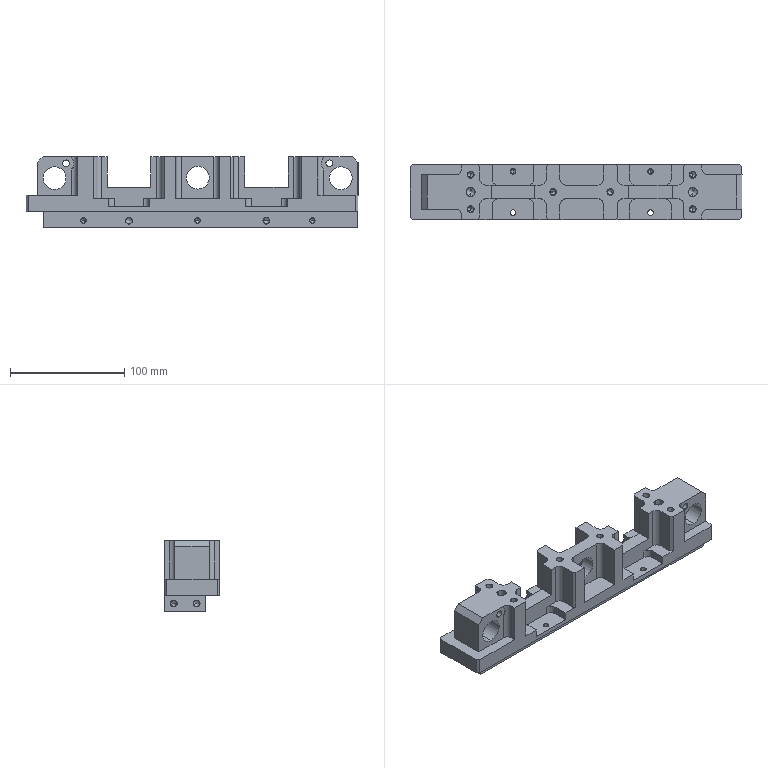Part | STEP file | J454-EBZ05-11-03-Part-1 | 1 solid | 274 faces | box 290 x 48 x 62 mm | volume 468483 mm3 | cylinder 128 | plane 104 | cone 42 | commonest cylinder face diameters 6 x30 10 x24 5.1 x22 5 x14 4.2 x10 20 x6